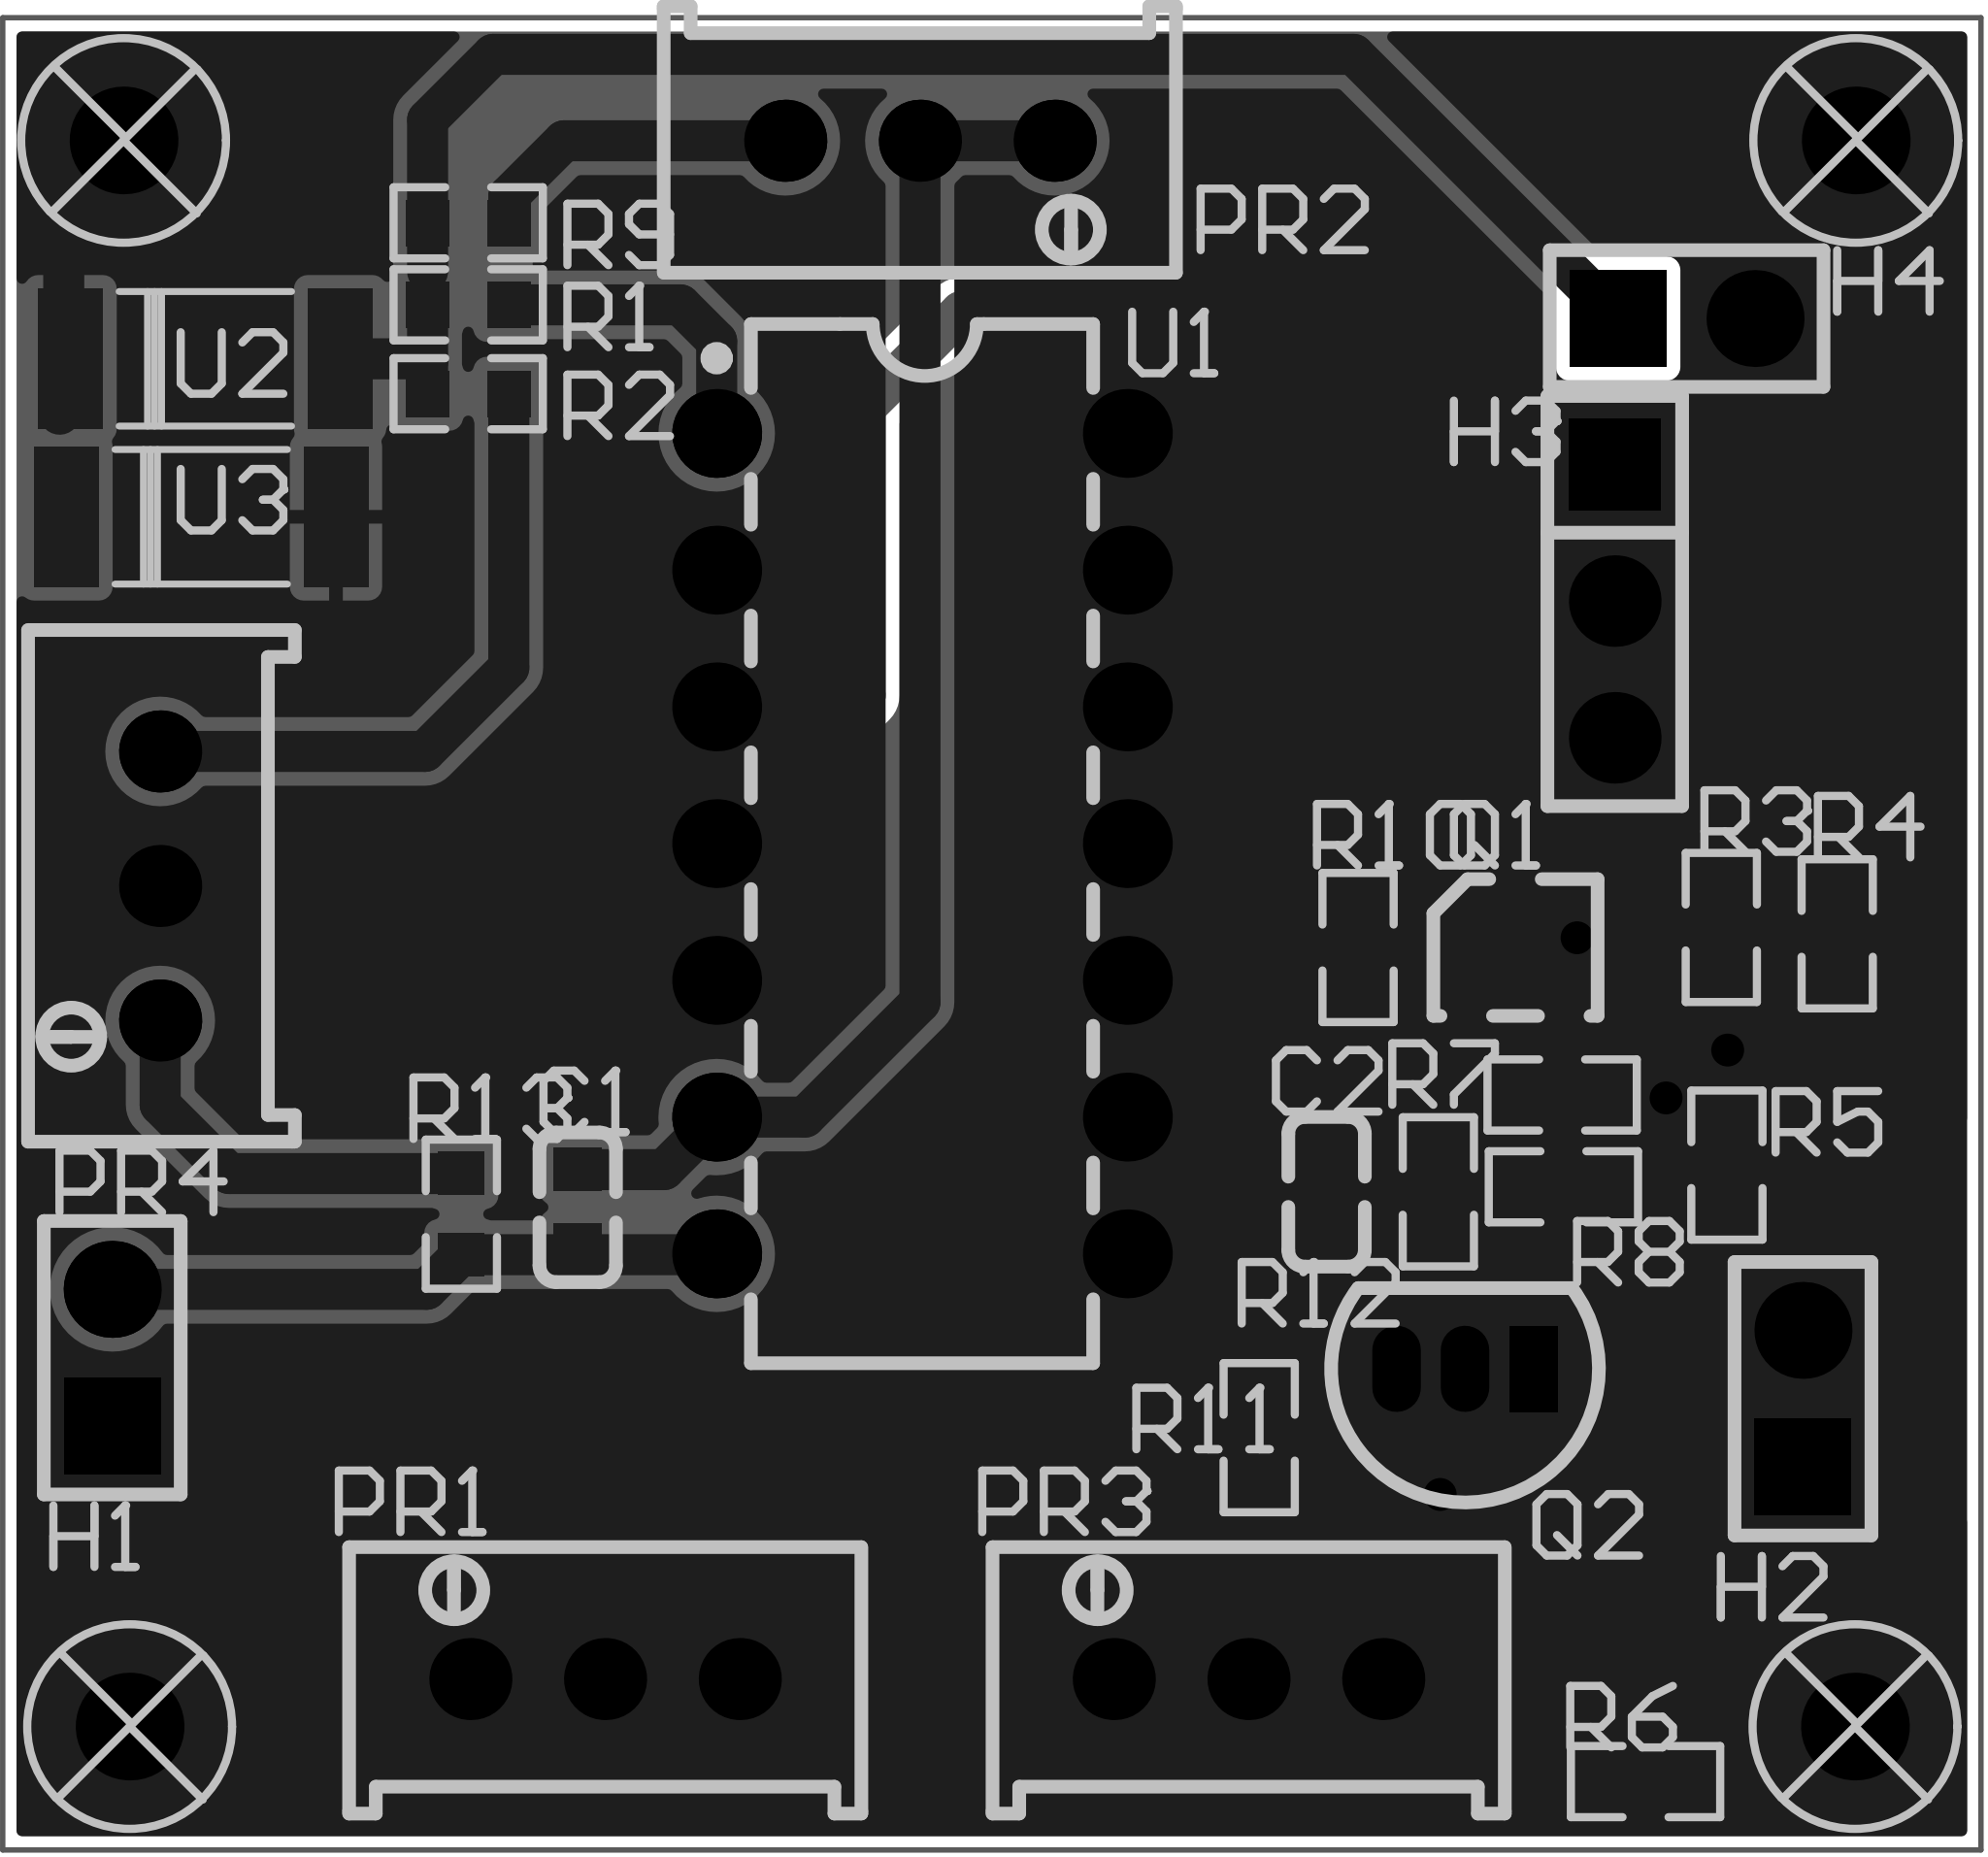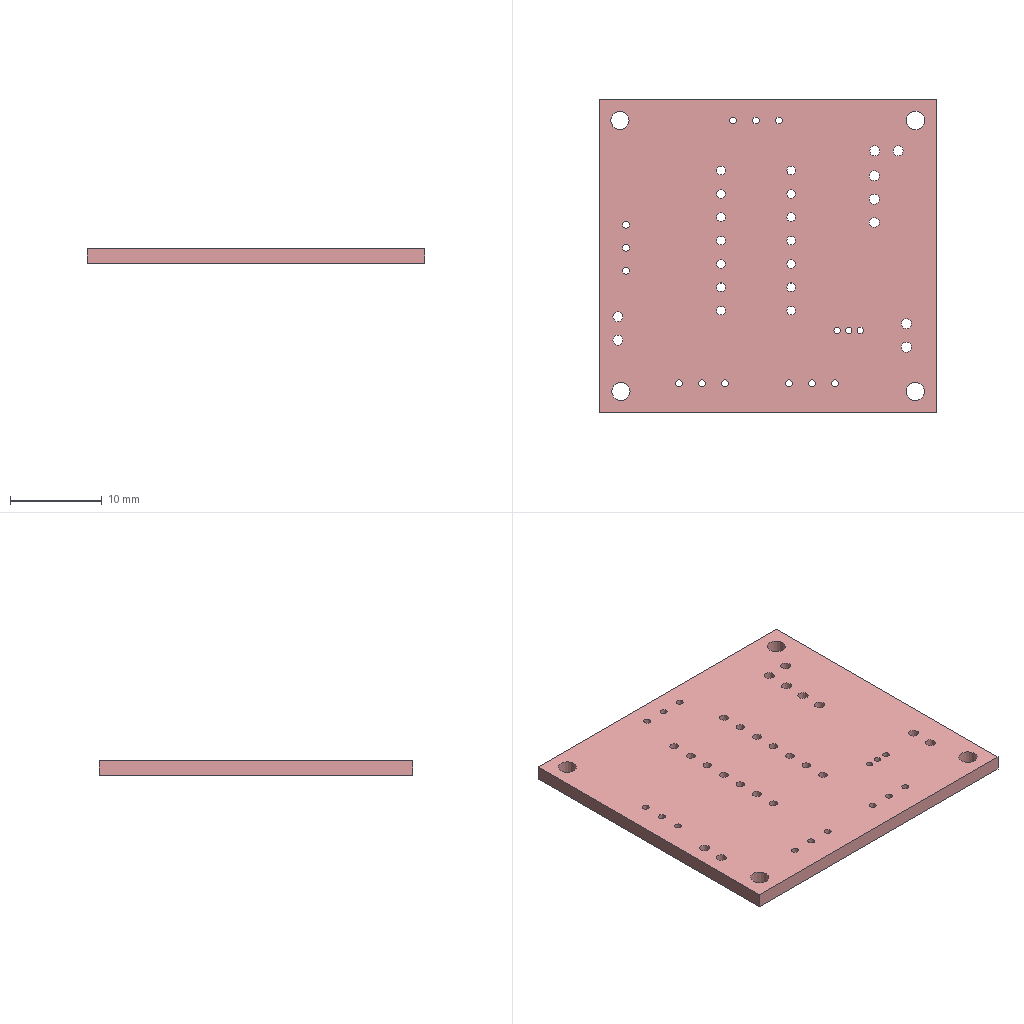Circuit board layout | Altium Designer | box 36.7 x 34 x 1.6 mm
Layer stack:
# Altium Designer layer stack of  (unit mm; dielectric type: 0 none, 1 core, 2 prepreg, 3 surface material)
index,name,kind,layer,copper_thickness_mm,dielectric_type,dielectric_thickness_mm,dielectric_material,dielectric_constant
0,Top Paste Mask Layer,other,,,,,,
1,Top Silkscreen Layer,other,,,,,,
2,Top Solder Mask Layer,dielectric,,,3,0.01,,3.3
3,Top Layer,copper,Top Layer,0.035,,,,
4,Dielectric1,dielectric,,,3,1.51,FR4,4.5
5,Bottom Layer,copper,Bottom Layer,0.035,,,,
6,Bottom Solder Mask Layer,dielectric,,,3,0.01,,3.3
7,Bottom Silkscreen Layer,other,,,,,,
8,Bottom Paste Mask Layer,other,,,,,,
# drill layer pairs: low layer,high layer
drill_pair,Top Layer,Bottom Layer
Part placement:
Designator,Comment,Layer,Footprint,Center-X(mm),Center-Y(mm),Rotation
C1,100nF,TopLayer,C0603,88.519,90.424,90
C2,100pF,TopLayer,C0603,102.413,90.712,270
H1,,TopLayer,HDR-TH_2P-P2.54-V-M-1,79.883,87.63,90
H2,,TopLayer,HDR-TH_2P-P2.54-V-M-1,111.252,86.868,90
H4,,TopLayer,HDR-TH_2P-P2.54-V-M-1,109.093,106.934,0
PR1,10kΩ,TopLayer,R_3296,89.027,81.661,0
PR2,100kΩ,TopLayer,R_3296,94.869,110.236,180
PR3,500,TopLayer,R_3296,100.965,81.661,0
PR4,5kΩ,TopLayer,R_3296,80.772,96.393,90
Q1,2N222,TopLayer,SMD_3-L3.0-W2.5_JANTXV2N2222AUB,105.918,95.25,0
Q2,2N3391A,TopLayer,TO-92-3_L4.9-W3.7-P1.27-L,104.982,87.423,180
R1,1kΩ,TopLayer,R0603,86.487,107.188,0
R2,20kΩ,TopLayer,R0603,86.487,105.537,0
R3,2.2K,TopLayer,R0603,109.737,95.622,90
R4,220,TopLayer,R0603,111.887,95.504,90
R5,390,TopLayer,R0603,109.84,91.208,270
R6,20K,TopLayer,R0603,108.331,79.756,180
R7,4.7K,TopLayer,R0603,106.784,92.511,0
R8,4.7K,TopLayer,R0603,106.807,90.805,0
R9,4.7K,TopLayer,R0603,86.487,108.712,0
R10,4.7K,TopLayer,R0603,102.997,95.25,270
R11,220,TopLayer,R0603,101.163,86.145,90
R12,4.7K,TopLayer,R0603,104.487,90.712,90
R13,20kΩ,TopLayer,R0603,86.36,90.297,270
U1,LM324N/PB,TopLayer,PDIP-14_L19.2-W6.6-P2.54-LS7.6-BL,94.907,97.18,270
U2,稳压管474536VSMA,TopLayer,LL-41_L5.0-W2.5-RD,81.61,106.185,0
U3,稳压管474536VSMA,TopLayer,LL-41_L5.0-W2.5-RD,81.534,103.251,0
H3,,TopLayer,HDR-TH_3P-P2.54-V-M,107.76,101.686,270
SCREW1,,TopLayer,M2螺丝,80.206,80.778,0
SCREW2,,TopLayer,M2螺丝,112.217,80.778,0
SCREW3,,TopLayer,M2螺丝,80.093,110.242,0
SCREW4,,TopLayer,M2螺丝,112.231,110.242,0
Pad and via stacks:
# Altium Designer via and pad stacks of  (unit mm). Each distinct definition once, with the count of objects using it.
# via: kind,start_layer,end_layer,hole_mm,diameter_mm,mode(0 simple;1 top-mid-bottom;2 full stack),diameter_per_layer,count,example_net
# pad: kind,layer,hole_mm,hole_type(0 round;1 square;2 slot),plating,top_size,top_shape(1 round;2 rect;3 octagon;9 rounded rect),mid_size,bottom_size,mode,footprint,size_per_layer,count,example
pad,Top Layer,0,0,plated,0.8x0.9,2,0.8x0.9,0.8x0.9,0,C0603,,4,C1.2
pad,Top Layer,0,0,plated,0.51x0.8,2,0.51x0.8,0.51x0.8,0,SMD_3-L3.0-W2.5_JANTXV2N2222AUB,,3,Q1.3
pad,Top Layer,0,0,plated,0.8065x0.864,2,0.8065x0.864,0.8065x0.864,0,R0603,,26,R1.2
pad,Top Layer,0,0,plated,1.2x2.6,2,1.2x2.6,1.2x2.6,0,LL-41_L5.0-W2.5-RD,,4,U2.2
pad,Multi-Layer,1.1,0,plated,1.8x1.8,1,1.8x1.8,1.8x1.8,0,HDR-TH_2P-P2.54-V-M-1,,3,H1.2
pad,Multi-Layer,1.1,0,plated,1.8x1.8,2,1.8x1.8,1.8x1.8,0,HDR-TH_2P-P2.54-V-M-1,,3,H1.1
pad,Multi-Layer,0.762,0,plated,1.524x1.524,1,1.524x1.524,1.524x1.524,0,R_3296,,12,PR1.2
pad,Multi-Layer,0.7,0,plated,0.9x1.6,1,0.9x1.6,0.9x1.6,0,TO-92-3_L4.9-W3.7-P1.27-L,,2,Q2.3
pad,Multi-Layer,0.7,0,plated,0.9x1.6,2,0.9x1.6,0.9x1.6,0,TO-92-3_L4.9-W3.7-P1.27-L,,1,Q2.1
pad,Multi-Layer,0.95,0,plated,1.65x1.65,1,1.65x1.65,1.65x1.65,0,PDIP-14_L19.2-W6.6-P2.54-LS7.6-BL,,14,U1.1
pad,Multi-Layer,1.1,0,plated,1.7x1.7,2,1.7x1.7,1.7x1.7,0,HDR-TH_3P-P2.54-V-M,,1,H3.1
pad,Multi-Layer,1.1,0,plated,1.7x1.7,1,1.7x1.7,1.7x1.7,0,HDR-TH_3P-P2.54-V-M,,2,H3.2
pad,Multi-Layer,2,0,plated,2x2,1,2x2,2x2,0,M2\u00C2\u00DD\u00CB\u00BF,,4,SCREW1.1
via,Top Layer,Bottom Layer,0.3048,0.61,0,,4,$1N44
Copper pours:
name,layer,net,type(0 solid;1 hatched;2 none)
Top Layer-GND,Top Layer,GND,0
Bottom Layer-GND,Bottom Layer,GND,0